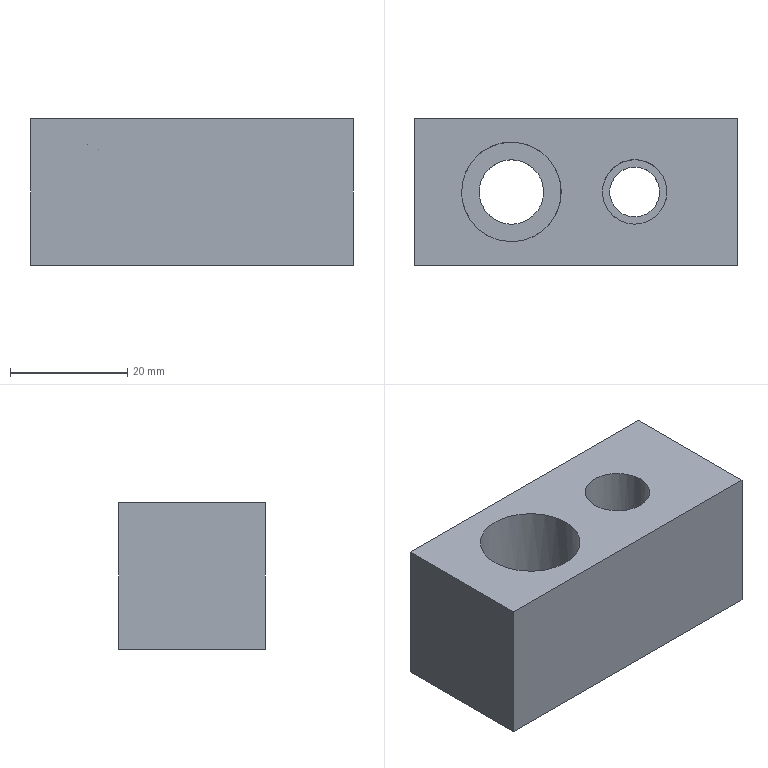Part | STEP file | lll_id3886_x_t | 1 solid | 12 faces | box 55 x 25 x 25 mm | volume 28499 mm3 | plane 8 | cylinder 4 | commonest cylinder face diameters 11 x2 8.5 x1 17 x1
STEP:
#1=CARTESIAN_POINT('',(1318.474,-86.93,-48.));
#2=VERTEX_POINT('',#1);
#3=CARTESIAN_POINT('',(1318.474,-86.93,-23.));
#4=VERTEX_POINT('',#3);
#5=CARTESIAN_POINT('',(1318.474,-86.93,-48.));
#6=DIRECTION('',(0.,0.,1.));
#7=VECTOR('',#6,1.);
#8=LINE('',#5,#7);
#9=EDGE_CURVE('',#2,#4,#8,.T.);
#10=ORIENTED_EDGE('',*,*,#9,.F.);
#11=CARTESIAN_POINT('',(1263.474,-86.93,-48.));
#12=VERTEX_POINT('',#11);
#13=CARTESIAN_POINT('',(1300.974,-86.93,-48.));
#14=DIRECTION('',(1.,0.,0.));
#15=VECTOR('',#14,1.);
#16=LINE('',#13,#15);
#17=EDGE_CURVE('',#12,#2,#16,.T.);
#18=ORIENTED_EDGE('',*,*,#17,.F.);
#19=CARTESIAN_POINT('',(1263.474,-86.93,-23.));
#20=VERTEX_POINT('',#19);
#21=CARTESIAN_POINT('',(1263.474,-86.93,-48.));
#22=DIRECTION('',(0.,0.,1.));
#23=VECTOR('',#22,1.);
#24=LINE('',#21,#23);
#25=EDGE_CURVE('',#12,#20,#24,.T.);
#26=ORIENTED_EDGE('',*,*,#25,.T.);
#27=CARTESIAN_POINT('',(1215.974,-86.93,-23.));
#28=DIRECTION('',(-1.,0.,0.));
#29=VECTOR('',#28,1.);
#30=LINE('',#27,#29);
#31=EDGE_CURVE('',#4,#20,#30,.T.);
#32=ORIENTED_EDGE('',*,*,#31,.F.);
#33=EDGE_LOOP('',(#10,#18,#26,#32));
#34=FACE_OUTER_BOUND('',#33,.T.);
#35=CARTESIAN_POINT('',(1300.974,-86.93,-48.));
#36=DIRECTION('',(0.,1.,0.));
#37=DIRECTION('',(0.,0.,-1.));
#38=AXIS2_PLACEMENT_3D('',#35,#36,#37);
#39=PLANE('',#38);
#40=ADVANCED_FACE('',(#34),#39,.T.);
#41=CARTESIAN_POINT('',(1279.974,-104.93,-35.));
#42=VERTEX_POINT('',#41);
#43=CARTESIAN_POINT('',(1279.974,-99.43,-35.));
#44=DIRECTION('',(0.,0.,-1.));
#45=DIRECTION('',(0.,-1.,0.));
#46=AXIS2_PLACEMENT_3D('',#43,#44,#45);
#47=CIRCLE('',#46,5.5);
#48=EDGE_CURVE('',#42,#42,#47,.T.);
#49=ORIENTED_EDGE('',*,*,#48,.T.);
#50=EDGE_LOOP('',(#49));
#51=FACE_BOUND('',#50,.T.);
#52=CARTESIAN_POINT('',(1279.974,-107.93,-35.));
#53=VERTEX_POINT('',#52);
#54=CARTESIAN_POINT('',(1279.974,-99.43,-35.));
#55=DIRECTION('',(0.,0.,-1.));
#56=DIRECTION('',(0.,-1.,0.));
#57=AXIS2_PLACEMENT_3D('',#54,#55,#56);
#58=CIRCLE('',#57,8.5);
#59=EDGE_CURVE('',#53,#53,#58,.T.);
#60=ORIENTED_EDGE('',*,*,#59,.F.);
#61=EDGE_LOOP('',(#60));
#62=FACE_BOUND('',#61,.T.);
#63=CARTESIAN_POINT('',(1315.474,-99.43,-35.));
#64=DIRECTION('',(0.,0.,-1.));
#65=DIRECTION('',(-1.,0.,0.));
#66=AXIS2_PLACEMENT_3D('',#63,#64,#65);
#67=PLANE('',#66);
#68=ADVANCED_FACE('',(#51,#62),#67,.F.);
#69=CARTESIAN_POINT('',(1300.974,-103.68,-36.));
#70=VERTEX_POINT('',#69);
#71=CARTESIAN_POINT('',(1300.974,-99.43,-36.));
#72=DIRECTION('',(0.,0.,-1.));
#73=DIRECTION('',(0.,-1.,0.));
#74=AXIS2_PLACEMENT_3D('',#71,#72,#73);
#75=CIRCLE('',#74,4.25);
#76=EDGE_CURVE('',#70,#70,#75,.T.);
#77=ORIENTED_EDGE('',*,*,#76,.T.);
#78=EDGE_LOOP('',(#77));
#79=FACE_BOUND('',#78,.T.);
#80=CARTESIAN_POINT('',(1300.974,-104.93,-36.));
#81=VERTEX_POINT('',#80);
#82=CARTESIAN_POINT('',(1300.974,-99.43,-36.));
#83=DIRECTION('',(0.,0.,-1.));
#84=DIRECTION('',(0.,-1.,0.));
#85=AXIS2_PLACEMENT_3D('',#82,#83,#84);
#86=CIRCLE('',#85,5.5);
#87=EDGE_CURVE('',#81,#81,#86,.T.);
#88=ORIENTED_EDGE('',*,*,#87,.F.);
#89=EDGE_LOOP('',(#88));
#90=FACE_BOUND('',#89,.T.);
#91=CARTESIAN_POINT('',(1300.974,-99.43,-36.));
#92=DIRECTION('',(0.,0.,-1.));
#93=DIRECTION('',(-1.,0.,0.));
#94=AXIS2_PLACEMENT_3D('',#91,#92,#93);
#95=PLANE('',#94);
#96=ADVANCED_FACE('',(#79,#90),#95,.F.);
#97=CARTESIAN_POINT('',(1263.474,-111.93,-48.));
#98=VERTEX_POINT('',#97);
#99=CARTESIAN_POINT('',(1263.474,-111.93,-23.));
#100=VERTEX_POINT('',#99);
#101=CARTESIAN_POINT('',(1263.474,-111.93,-48.));
#102=DIRECTION('',(0.,0.,1.));
#103=VECTOR('',#102,1.);
#104=LINE('',#101,#103);
#105=EDGE_CURVE('',#98,#100,#104,.T.);
#106=ORIENTED_EDGE('',*,*,#105,.F.);
#107=CARTESIAN_POINT('',(1318.474,-111.93,-48.));
#108=VERTEX_POINT('',#107);
#109=CARTESIAN_POINT('',(1300.974,-111.93,-48.));
#110=DIRECTION('',(-1.,0.,0.));
#111=VECTOR('',#110,1.);
#112=LINE('',#109,#111);
#113=EDGE_CURVE('',#108,#98,#112,.T.);
#114=ORIENTED_EDGE('',*,*,#113,.F.);
#115=CARTESIAN_POINT('',(1318.474,-111.93,-23.));
#116=VERTEX_POINT('',#115);
#117=CARTESIAN_POINT('',(1318.474,-111.93,-48.));
#118=DIRECTION('',(0.,0.,1.));
#119=VECTOR('',#118,1.);
#120=LINE('',#117,#119);
#121=EDGE_CURVE('',#108,#116,#120,.T.);
#122=ORIENTED_EDGE('',*,*,#121,.T.);
#123=CARTESIAN_POINT('',(1215.974,-111.93,-23.));
#124=DIRECTION('',(1.,0.,0.));
#125=VECTOR('',#124,1.);
#126=LINE('',#123,#125);
#127=EDGE_CURVE('',#100,#116,#126,.T.);
#128=ORIENTED_EDGE('',*,*,#127,.F.);
#129=EDGE_LOOP('',(#106,#114,#122,#128));
#130=FACE_OUTER_BOUND('',#129,.T.);
#131=CARTESIAN_POINT('',(1300.974,-111.93,-48.));
#132=DIRECTION('',(0.,-1.,0.));
#133=DIRECTION('',(0.,0.,1.));
#134=AXIS2_PLACEMENT_3D('',#131,#132,#133);
#135=PLANE('',#134);
#136=ADVANCED_FACE('',(#130),#135,.T.);
#137=CARTESIAN_POINT('',(1263.474,-221.93,-23.));
#138=DIRECTION('',(0.,-1.,0.));
#139=VECTOR('',#138,1.);
#140=LINE('',#137,#139);
#141=EDGE_CURVE('',#20,#100,#140,.T.);
#142=ORIENTED_EDGE('',*,*,#141,.F.);
#143=ORIENTED_EDGE('',*,*,#25,.F.);
#144=CARTESIAN_POINT('',(1263.474,-99.43,-48.));
#145=DIRECTION('',(0.,1.,0.));
#146=VECTOR('',#145,1.);
#147=LINE('',#144,#146);
#148=EDGE_CURVE('',#98,#12,#147,.T.);
#149=ORIENTED_EDGE('',*,*,#148,.F.);
#150=ORIENTED_EDGE('',*,*,#105,.T.);
#151=EDGE_LOOP('',(#142,#143,#149,#150));
#152=FACE_OUTER_BOUND('',#151,.T.);
#153=CARTESIAN_POINT('',(1263.474,-99.43,-48.));
#154=DIRECTION('',(-1.,0.,0.));
#155=DIRECTION('',(0.,0.,1.));
#156=AXIS2_PLACEMENT_3D('',#153,#154,#155);
#157=PLANE('',#156);
#158=ADVANCED_FACE('',(#152),#157,.T.);
#159=CARTESIAN_POINT('',(1318.474,-99.43,-23.));
#160=DIRECTION('',(0.,1.,0.));
#161=VECTOR('',#160,1.);
#162=LINE('',#159,#161);
#163=EDGE_CURVE('',#116,#4,#162,.T.);
#164=ORIENTED_EDGE('',*,*,#163,.F.);
#165=ORIENTED_EDGE('',*,*,#121,.F.);
#166=CARTESIAN_POINT('',(1318.474,-99.43,-48.));
#167=DIRECTION('',(0.,-1.,0.));
#168=VECTOR('',#167,1.);
#169=LINE('',#166,#168);
#170=EDGE_CURVE('',#2,#108,#169,.T.);
#171=ORIENTED_EDGE('',*,*,#170,.F.);
#172=ORIENTED_EDGE('',*,*,#9,.T.);
#173=EDGE_LOOP('',(#164,#165,#171,#172));
#174=FACE_OUTER_BOUND('',#173,.T.);
#175=CARTESIAN_POINT('',(1318.474,-99.43,-48.));
#176=DIRECTION('',(-1.,0.,0.));
#177=DIRECTION('',(0.,0.,1.));
#178=AXIS2_PLACEMENT_3D('',#175,#176,#177);
#179=PLANE('',#178);
#180=ADVANCED_FACE('',(#174),#179,.F.);
#181=CARTESIAN_POINT('',(1279.974,-104.93,-48.));
#182=VERTEX_POINT('',#181);
#183=CARTESIAN_POINT('',(1279.974,-99.43,-48.));
#184=DIRECTION('',(0.,0.,1.));
#185=DIRECTION('',(0.,-1.,0.));
#186=AXIS2_PLACEMENT_3D('',#183,#184,#185);
#187=CIRCLE('',#186,5.5);
#188=EDGE_CURVE('',#182,#182,#187,.T.);
#189=ORIENTED_EDGE('',*,*,#188,.F.);
#190=EDGE_LOOP('',(#189));
#191=FACE_BOUND('',#190,.T.);
#192=ORIENTED_EDGE('',*,*,#48,.F.);
#193=EDGE_LOOP('',(#192));
#194=FACE_BOUND('',#193,.T.);
#195=CARTESIAN_POINT('',(1279.974,-99.43,-78.));
#196=DIRECTION('',(0.,0.,-1.));
#197=DIRECTION('',(0.,-1.,0.));
#198=AXIS2_PLACEMENT_3D('',#195,#196,#197);
#199=CYLINDRICAL_SURFACE('',#198,5.5);
#200=ADVANCED_FACE('',(#191,#194),#199,.F.);
#201=CARTESIAN_POINT('',(1300.974,-103.68,-48.));
#202=VERTEX_POINT('',#201);
#203=CARTESIAN_POINT('',(1300.974,-99.43,-48.));
#204=DIRECTION('',(0.,0.,1.));
#205=DIRECTION('',(0.,-1.,0.));
#206=AXIS2_PLACEMENT_3D('',#203,#204,#205);
#207=CIRCLE('',#206,4.25);
#208=EDGE_CURVE('',#202,#202,#207,.T.);
#209=ORIENTED_EDGE('',*,*,#208,.F.);
#210=EDGE_LOOP('',(#209));
#211=FACE_BOUND('',#210,.T.);
#212=ORIENTED_EDGE('',*,*,#76,.F.);
#213=EDGE_LOOP('',(#212));
#214=FACE_BOUND('',#213,.T.);
#215=CARTESIAN_POINT('',(1300.974,-99.43,-78.));
#216=DIRECTION('',(0.,0.,-1.));
#217=DIRECTION('',(0.,-1.,0.));
#218=AXIS2_PLACEMENT_3D('',#215,#216,#217);
#219=CYLINDRICAL_SURFACE('',#218,4.25);
#220=ADVANCED_FACE('',(#211,#214),#219,.F.);
#221=ORIENTED_EDGE('',*,*,#17,.T.);
#222=ORIENTED_EDGE('',*,*,#170,.T.);
#223=ORIENTED_EDGE('',*,*,#113,.T.);
#224=ORIENTED_EDGE('',*,*,#148,.T.);
#225=EDGE_LOOP('',(#221,#222,#223,#224));
#226=FACE_BOUND('',#225,.T.);
#227=ORIENTED_EDGE('',*,*,#208,.T.);
#228=EDGE_LOOP('',(#227));
#229=FACE_BOUND('',#228,.T.);
#230=ORIENTED_EDGE('',*,*,#188,.T.);
#231=EDGE_LOOP('',(#230));
#232=FACE_BOUND('',#231,.T.);
#233=CARTESIAN_POINT('',(1300.974,-99.43,-48.));
#234=DIRECTION('',(0.,0.,-1.));
#235=DIRECTION('',(-1.,0.,0.));
#236=AXIS2_PLACEMENT_3D('',#233,#234,#235);
#237=PLANE('',#236);
#238=ADVANCED_FACE('',(#226,#229,#232),#237,.T.);
#239=ORIENTED_EDGE('',*,*,#59,.T.);
#240=EDGE_LOOP('',(#239));
#241=FACE_BOUND('',#240,.T.);
#242=CARTESIAN_POINT('',(1288.474,-99.43,-23.));
#243=VERTEX_POINT('',#242);
#244=CARTESIAN_POINT('',(1279.974,-99.43,-23.));
#245=DIRECTION('',(0.,0.,1.));
#246=DIRECTION('',(1.,0.,0.));
#247=AXIS2_PLACEMENT_3D('',#244,#245,#246);
#248=CIRCLE('',#247,8.5);
#249=EDGE_CURVE('',#243,#243,#248,.T.);
#250=ORIENTED_EDGE('',*,*,#249,.T.);
#251=EDGE_LOOP('',(#250));
#252=FACE_BOUND('',#251,.T.);
#253=CARTESIAN_POINT('',(1279.974,-99.43,-28.));
#254=DIRECTION('',(0.,0.,-1.));
#255=DIRECTION('',(0.,-1.,0.));
#256=AXIS2_PLACEMENT_3D('',#253,#254,#255);
#257=CYLINDRICAL_SURFACE('',#256,8.5);
#258=ADVANCED_FACE('',(#241,#252),#257,.F.);
#259=ORIENTED_EDGE('',*,*,#87,.T.);
#260=EDGE_LOOP('',(#259));
#261=FACE_BOUND('',#260,.T.);
#262=CARTESIAN_POINT('',(1306.474,-99.43,-23.));
#263=VERTEX_POINT('',#262);
#264=CARTESIAN_POINT('',(1300.974,-99.43,-23.));
#265=DIRECTION('',(0.,0.,1.));
#266=DIRECTION('',(1.,0.,0.));
#267=AXIS2_PLACEMENT_3D('',#264,#265,#266);
#268=CIRCLE('',#267,5.5);
#269=EDGE_CURVE('',#263,#263,#268,.T.);
#270=ORIENTED_EDGE('',*,*,#269,.T.);
#271=EDGE_LOOP('',(#270));
#272=FACE_BOUND('',#271,.T.);
#273=CARTESIAN_POINT('',(1300.974,-99.43,-28.));
#274=DIRECTION('',(0.,0.,-1.));
#275=DIRECTION('',(0.,-1.,0.));
#276=AXIS2_PLACEMENT_3D('',#273,#274,#275);
#277=CYLINDRICAL_SURFACE('',#276,5.5);
#278=ADVANCED_FACE('',(#261,#272),#277,.F.);
#279=ORIENTED_EDGE('',*,*,#31,.T.);
#280=ORIENTED_EDGE('',*,*,#141,.T.);
#281=ORIENTED_EDGE('',*,*,#127,.T.);
#282=ORIENTED_EDGE('',*,*,#163,.T.);
#283=EDGE_LOOP('',(#279,#280,#281,#282));
#284=FACE_BOUND('',#283,.T.);
#285=ORIENTED_EDGE('',*,*,#269,.F.);
#286=EDGE_LOOP('',(#285));
#287=FACE_BOUND('',#286,.T.);
#288=ORIENTED_EDGE('',*,*,#249,.F.);
#289=EDGE_LOOP('',(#288));
#290=FACE_BOUND('',#289,.T.);
#291=CARTESIAN_POINT('',(1215.974,-221.93,-23.));
#292=DIRECTION('',(0.,0.,1.));
#293=DIRECTION('',(0.,1.,0.));
#294=AXIS2_PLACEMENT_3D('',#291,#292,#293);
#295=PLANE('',#294);
#296=ADVANCED_FACE('',(#284,#287,#290),#295,.T.);
#297=CLOSED_SHELL('',(#40,#68,#96,#136,#158,#180,#200,#220,#238,#258,#278,#296));
#298=MANIFOLD_SOLID_BREP('',#297);
#299=(LENGTH_UNIT()NAMED_UNIT(*)SI_UNIT(.MILLI.,.METRE.));
#300=UNCERTAINTY_MEASURE_WITH_UNIT(LENGTH_MEASURE(0.00002),#299,'','');
#301=(NAMED_UNIT(*)PLANE_ANGLE_UNIT()SI_UNIT($,.RADIAN.));
#302=PLANE_ANGLE_MEASURE_WITH_UNIT(PLANE_ANGLE_MEASURE(0.01745),#301);
#303=DIMENSIONAL_EXPONENTS(0.,0.,0.,0.,0.,0.,0.);
#304=(CONVERSION_BASED_UNIT('DEGREE',#302)NAMED_UNIT(#303)PLANE_ANGLE_UNIT());
#305=(NAMED_UNIT(*)SI_UNIT($,.STERADIAN.)SOLID_ANGLE_UNIT());
#306=(GEOMETRIC_REPRESENTATION_CONTEXT(3)GLOBAL_UNCERTAINTY_ASSIGNED_CONTEXT((#300))GLOBAL_UNIT_ASSIGNED_CONTEXT((#299,#304,#305))REPRESENTATION_CONTEXT('',''));
#307=ADVANCED_BREP_SHAPE_REPRESENTATION('',(#298),#306);